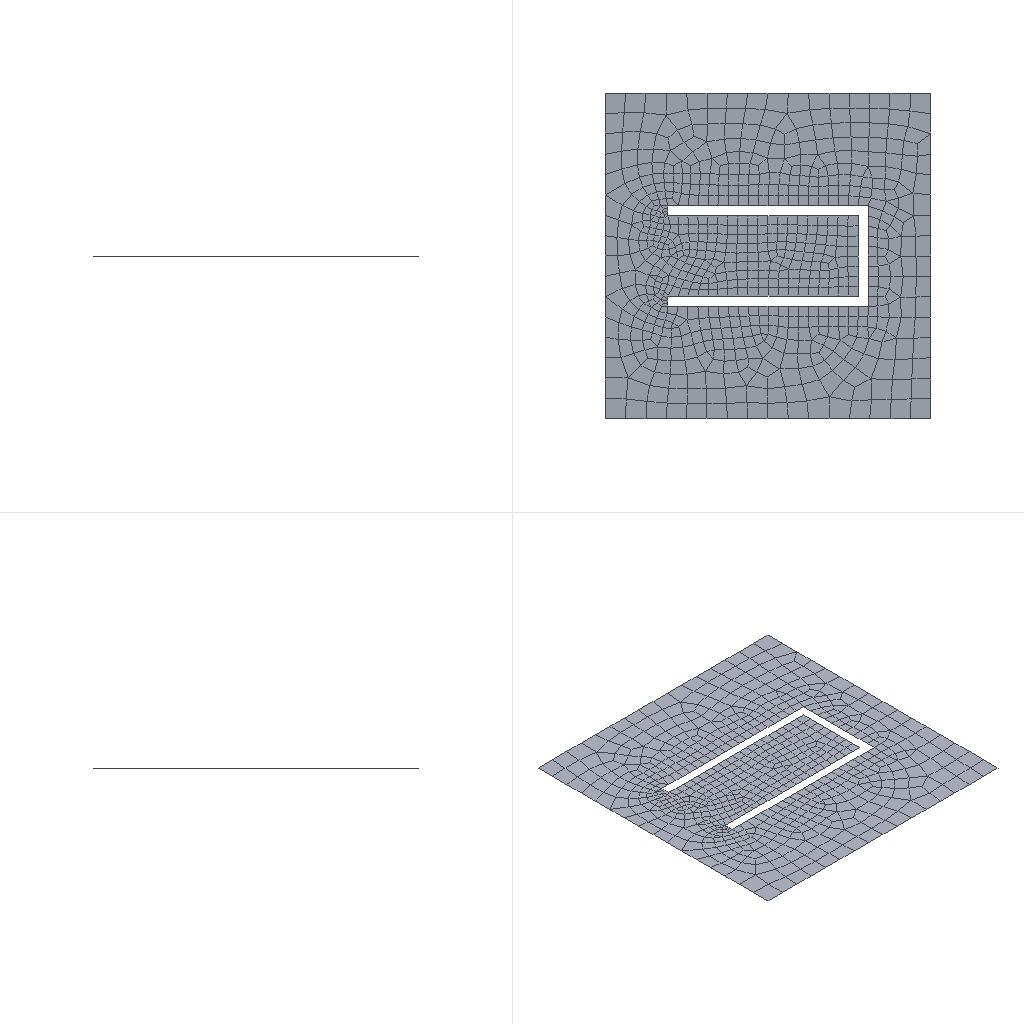Simulation study | abaqus
Set-up summary:
category,name,step,type,value,unit,region
solver,abaqus
solver,version,,,Abaqus/Explicit 2020
units,not stated in the deck,,not stated
analysis,deck,,transient,transient
load_step,Step-1,Step-1,transient
load_step,requested,,,1
mesh,nodes,,,8020
mesh,elements,,,7660
element_type,S3R,,shell,14
element_type,S4R,,shell,706
element_type,MASS,,point,3
element_type,R3D3,,rigid,158
element_type,R3D4,,rigid,6776
element_type,ROTARYI,,mass,3
load,load commands in deck,,count,2
bc,support commands in deck,,count,14
material,CHUNTIE N,,in results
check,setup vs results,,match,"per instance, exact: element labels, types and connectivity; labels of the nodes the elements use; coordinates of those nodes at SINGLE_PRECISION in 4 of 4 instance(s)"
Abaqus input file, long lists of numbers shortened:
*Heading
** Job name: Job-3 Model name: Model-1
** Generated by: Abaqus/CAE 2020
*Preprint, echo=NO, model=NO, history=NO, contact=NO
**
** PARTS
**
*Part, name=blank
*Node
      1,        1.625,       -1.625,   -2.15
      2,       -1.625,       -1.625,   -2.15
** (795 more lines like these left out)
*Element, type=S3R
 1, 518, 583, 564
 2, 455, 283, 378
** (12 more lines like these left out)
*Element, type=S4R
 15, 701, 710, 721, 713
 16, 190, 283, 455, 377
** (704 more lines like these left out)
*Nset, nset=Set-1, generate
   1,  797,    1
*Elset, elset=Set-1, generate
   1,  720,    1
** Section: Section-1
*Shell Section, elset=Set-1, material="chuntie n"
0.3, 5
*End Part
**
*Part, name=flange
*Node
      1, -0.8958, -0.4,  -1.009
      2,          -1., -0.4,          -1.
** (394 more lines like these left out)
*Element, type=R3D4
 1,   1,  11, 118,  36
 2,  11,  12, 119, 118
** (348 more lines like these left out)
*Node
    397,  0.8738,           0.,  -1.305
*Nset, nset=flange-RefPt_, internal
397,
*Nset, nset=Set-7
 397,
*Elset, elset=flange, generate
   1,  350,    1
*Element, type=MASS, elset=Set-7_Inertia-1_MASS_
351, 397
*Mass, elset=Set-7_Inertia-1_MASS_
1.,
*Element, type=ROTARYI, elset=Set-7_Inertia-1_ROTI_
352, 397
*Rotary Inertia, elset=Set-7_Inertia-1_ROTI_
1., 1., 1., 0., 0., 0.
*End Part
**
*Part, name=pad
*Node
      1,   1.55,        -1.75,  -1.67
      2,   1.45,        -1.75,  -1.67
** (2352 more lines like these left out)
*Element, type=R3D3
 1, 1626,  170, 1607
 2, 1810, 1799,  354
** (68 more lines like these left out)
*Element, type=R3D4
  71,  451, 2004,  502,   22
  72,  502, 2004, 2014,   88
** (2187 more lines like these left out)
*Node
   2355,        -1.75,           0.,  -1.67
*Nset, nset=pad-RefPt_, internal
2355,
*Nset, nset=Set-3
 2355,
*Elset, elset=pad, generate
    1,  2259,     1
*Element, type=MASS, elset=Set-3_Inertia-1_MASS_
2260, 2355
*Mass, elset=Set-3_Inertia-1_MASS_
1.,
*Element, type=ROTARYI, elset=Set-3_Inertia-1_ROTI_
2261, 2355
*Rotary Inertia, elset=Set-3_Inertia-1_ROTI_
1., 1., 1., 0., 0., 0.
*End Part
**
*Part, name=post
*Node
      1,  -0.9479,  0.4,  -2.305
      2,  -0.9479, -0.4,  -2.305
** (4468 more lines like these left out)
*Element, type=R3D4
 1,   1,  19, 487,  74
 2,  19,  20, 488, 487
** (4235 more lines like these left out)
*Element, type=R3D3
1205, 3115, 3067, 1684
1206, 3394, 1657, 3207
** (86 more lines like these left out)
*Node
   4471,          -2.,           0.,  -2.3
*Nset, nset=post-RefPt_, internal
4471,
*Nset, nset=Set-5
 4471,
*Elset, elset=post, generate
    1,  4325,     1
*Element, type=MASS, elset=Set-5_Inertia-1_MASS_
4326, 4471
*Mass, elset=Set-5_Inertia-1_MASS_
1.,
*Element, type=ROTARYI, elset=Set-5_Inertia-1_ROTI_
4327, 4471
*Rotary Inertia, elset=Set-5_Inertia-1_ROTI_
1., 1., 1., 0., 0., 0.
*End Part
**
**
** ASSEMBLY
**
*Assembly, name=Assembly
**
*Instance, name=post-1, part=post
*End Instance
**
*Instance, name=flange-1, part=flange
*End Instance
**
*Instance, name=pad-1, part=pad
          0.,           0., -0.33
*End Instance
**
*Instance, name=blank-1, part=blank
*End Instance
**
*Nset, nset=Set-1, instance=blank-1, generate
   1,  797,    1
*Elset, elset=Set-1, instance=blank-1, generate
   1,  720,    1
*Nset, nset=Set-2, instance=pad-1, generate
    1,  2354,     1
*Elset, elset=Set-2, instance=pad-1, generate
    1,  2259,     1
*Nset, nset=_PickedSet14, internal, instance=pad-1
   22,   23,   45,   67,  100,  101,  107,  119, 2355
*Nset, nset=_PickedSet15, internal, instance=post-1, generate
    1,  4470,     1
*Elset, elset=_PickedSet15, internal, instance=post-1, generate
    1,  4325,     1
*Nset, nset=_PickedSet16, internal, instance=pad-1, generate
    1,  2354,     1
*Elset, elset=_PickedSet16, internal, instance=pad-1, generate
    1,  2259,     1
*Nset, nset=_PickedSet17, internal, instance=flange-1, generate
   1,  397,    1
*Elset, elset=_PickedSet17, internal, instance=flange-1, generate
   1,  350,    1
*Rigid Body, ref node=post-1.post-RefPt_, elset=post-1.post
*Rigid Body, ref node=flange-1.flange-RefPt_, elset=flange-1.flange
*Rigid Body, ref node=pad-1.pad-RefPt_, elset=pad-1.pad
*End Assembly
*Amplitude, name=Amp-1
             0.,              0.,             0.2,              1.
**
** MATERIALS
**
*Material, name="chuntie n"
*Density
 7.875e-09,
*Elastic
80650., 0.291
*Plastic
   98.45,   0.
 207.085, 0.02
 222.526, 0.04
 232.557, 0.06
 240.162, 0.08
 246.357,  0.1
 251.619, 0.12
 256.214, 0.14
 260.305, 0.16
  267.38,  0.2
 281.038,  0.3
 291.392,  0.4
 299.826,  0.5
  306.99,  0.6
**
** INTERACTION PROPERTIES
**
*Surface Interaction, name=IntProp-1
*Friction
0.,
**
** BOUNDARY CONDITIONS
**
** Name: BC-1 Type: Symmetry/Antisymmetry/Encastre
*Boundary
_PickedSet15, ENCASTRE
** Name: BC-2 Type: Symmetry/Antisymmetry/Encastre
*Boundary
_PickedSet16, ENCASTRE
** Name: BC-3 Type: Displacement/Rotation
*Boundary
_PickedSet17, 1, 1
_PickedSet17, 2, 2
_PickedSet17, 3, 3
_PickedSet17, 4, 4
_PickedSet17, 5, 5
_PickedSet17, 6, 6
** ----------------------------------------------------------------
**
** STEP: Step-1
**
*Step, name=Step-1, nlgeom=YES
*Dynamic, Explicit
, 0.2
*Bulk Viscosity
0.06, 1.2
** Mass Scaling: Semi-Automatic
**               Whole Model
*Fixed Mass Scaling, factor=5.
**
** BOUNDARY CONDITIONS
**
** Name: BC-3 Type: Displacement/Rotation
*Boundary, amplitude=Amp-1
_PickedSet17, 1, 1
_PickedSet17, 2, 2
_PickedSet17, 3, 3, -1.
_PickedSet17, 4, 4
_PickedSet17, 5, 5
_PickedSet17, 6, 6
**
** LOADS
**
** Name: Load-1   Type: Concentrated force
*Cload
_PickedSet14, 3, -2000.
**
** INTERACTIONS
**
** Interaction: Int-1
*Contact, op=NEW
*Contact Inclusions, ALL EXTERIOR
*Contact Property Assignment
 ,  , IntProp-1
**
** OUTPUT REQUESTS
**
*Restart, write, number interval=1, time marks=NO
**
** FIELD OUTPUT: F-Output-1
**
*Output, field, variable=PRESELECT
**
** HISTORY OUTPUT: H-Output-1
**
*Output, history, variable=PRESELECT
*End Step
Results summary:
result,step,Step-1,partial,increments=7757936 time=0.0878/0.2
result,analysis,,,transient
result,last_loadstep,,,1
result,primary field,,,"U, UR"
result,reaction total,,FX,0.0,model units
result,reaction total,,FY,0.0,model units
result,reaction total,,FZ,16000.0,model units